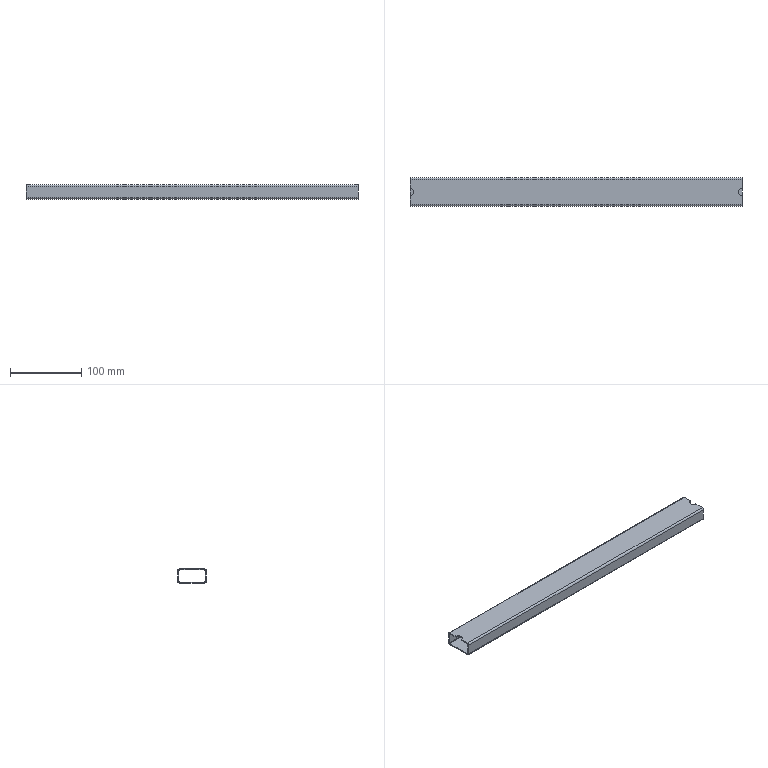Part | STEP file | 6150505 | 1 solid | 20 faces | box 465 x 40 x 20 mm | volume 77302 mm3 | plane 10 | cylinder 10 | commonest cylinder face diameters 2 x4 5 x4 10 x2
STEP:
#1=CARTESIAN_POINT('',(232.5,-5.,10.));
#2=VERTEX_POINT('',#1);
#3=CARTESIAN_POINT('',(232.5,-17.5,10.));
#4=VERTEX_POINT('',#3);
#5=CARTESIAN_POINT('',(232.5,20.,10.));
#6=DIRECTION('',(0.,-1.,0.));
#7=VECTOR('',#6,1000.);
#8=LINE('',#5,#7);
#9=EDGE_CURVE('',#2,#4,#8,.T.);
#10=ORIENTED_EDGE('',*,*,#9,.F.);
#11=CARTESIAN_POINT('',(232.5,5.,10.));
#12=VERTEX_POINT('',#11);
#13=CARTESIAN_POINT('',(232.5,0.,10.));
#14=DIRECTION('',(0.,0.,1.));
#15=DIRECTION('',(-1.,0.,0.));
#16=AXIS2_PLACEMENT_3D('',#13,#14,#15);
#17=CIRCLE('',#16,5.);
#18=EDGE_CURVE('',#12,#2,#17,.T.);
#19=ORIENTED_EDGE('',*,*,#18,.F.);
#20=CARTESIAN_POINT('',(232.5,17.5,10.));
#21=VERTEX_POINT('',#20);
#22=CARTESIAN_POINT('',(232.5,20.,10.));
#23=DIRECTION('',(0.,-1.,0.));
#24=VECTOR('',#23,1000.);
#25=LINE('',#22,#24);
#26=EDGE_CURVE('',#21,#12,#25,.T.);
#27=ORIENTED_EDGE('',*,*,#26,.F.);
#28=CARTESIAN_POINT('',(-232.5,17.5,10.));
#29=VERTEX_POINT('',#28);
#30=CARTESIAN_POINT('',(232.5,17.5,10.));
#31=DIRECTION('',(-1.,0.,0.));
#32=VECTOR('',#31,1000.);
#33=LINE('',#30,#32);
#34=EDGE_CURVE('',#21,#29,#33,.T.);
#35=ORIENTED_EDGE('',*,*,#34,.T.);
#36=CARTESIAN_POINT('',(-232.5,5.,10.));
#37=VERTEX_POINT('',#36);
#38=CARTESIAN_POINT('',(-232.5,20.,10.));
#39=DIRECTION('',(0.,-1.,0.));
#40=VECTOR('',#39,1000.);
#41=LINE('',#38,#40);
#42=EDGE_CURVE('',#29,#37,#41,.T.);
#43=ORIENTED_EDGE('',*,*,#42,.T.);
#44=CARTESIAN_POINT('',(-232.5,-5.,10.));
#45=VERTEX_POINT('',#44);
#46=CARTESIAN_POINT('',(-232.5,0.,10.));
#47=DIRECTION('',(0.,0.,1.));
#48=DIRECTION('',(1.,0.,0.));
#49=AXIS2_PLACEMENT_3D('',#46,#47,#48);
#50=CIRCLE('',#49,5.);
#51=EDGE_CURVE('',#45,#37,#50,.T.);
#52=ORIENTED_EDGE('',*,*,#51,.F.);
#53=CARTESIAN_POINT('',(-232.5,-17.5,10.));
#54=VERTEX_POINT('',#53);
#55=CARTESIAN_POINT('',(-232.5,20.,10.));
#56=DIRECTION('',(0.,-1.,0.));
#57=VECTOR('',#56,1000.);
#58=LINE('',#55,#57);
#59=EDGE_CURVE('',#45,#54,#58,.T.);
#60=ORIENTED_EDGE('',*,*,#59,.T.);
#61=CARTESIAN_POINT('',(232.5,-17.5,10.));
#62=DIRECTION('',(1.,0.,0.));
#63=VECTOR('',#62,1000.);
#64=LINE('',#61,#63);
#65=EDGE_CURVE('',#54,#4,#64,.T.);
#66=ORIENTED_EDGE('',*,*,#65,.T.);
#67=EDGE_LOOP('',(#10,#19,#27,#35,#43,#52,#60,#66));
#68=FACE_OUTER_BOUND('',#67,.T.);
#69=CARTESIAN_POINT('',(232.5,20.,10.));
#70=DIRECTION('',(0.,0.,-1.));
#71=DIRECTION('',(0.,1.,0.));
#72=AXIS2_PLACEMENT_3D('',#69,#70,#71);
#73=PLANE('',#72);
#74=ADVANCED_FACE('',(#68),#73,.F.);
#75=CARTESIAN_POINT('',(232.5,-20.,7.5));
#76=VERTEX_POINT('',#75);
#77=CARTESIAN_POINT('',(232.5,-20.,-7.5));
#78=VERTEX_POINT('',#77);
#79=CARTESIAN_POINT('',(232.5,-20.,10.));
#80=DIRECTION('',(0.,0.,-1.));
#81=VECTOR('',#80,1000.);
#82=LINE('',#79,#81);
#83=EDGE_CURVE('',#76,#78,#82,.T.);
#84=ORIENTED_EDGE('',*,*,#83,.F.);
#85=CARTESIAN_POINT('',(-232.5,-20.,7.5));
#86=VERTEX_POINT('',#85);
#87=CARTESIAN_POINT('',(232.5,-20.,7.5));
#88=DIRECTION('',(-1.,0.,0.));
#89=VECTOR('',#88,1000.);
#90=LINE('',#87,#89);
#91=EDGE_CURVE('',#76,#86,#90,.T.);
#92=ORIENTED_EDGE('',*,*,#91,.T.);
#93=CARTESIAN_POINT('',(-232.5,-20.,-7.5));
#94=VERTEX_POINT('',#93);
#95=CARTESIAN_POINT('',(-232.5,-20.,10.));
#96=DIRECTION('',(0.,0.,-1.));
#97=VECTOR('',#96,1000.);
#98=LINE('',#95,#97);
#99=EDGE_CURVE('',#86,#94,#98,.T.);
#100=ORIENTED_EDGE('',*,*,#99,.T.);
#101=CARTESIAN_POINT('',(232.5,-20.,-7.5));
#102=DIRECTION('',(1.,0.,0.));
#103=VECTOR('',#102,1000.);
#104=LINE('',#101,#103);
#105=EDGE_CURVE('',#94,#78,#104,.T.);
#106=ORIENTED_EDGE('',*,*,#105,.T.);
#107=EDGE_LOOP('',(#84,#92,#100,#106));
#108=FACE_OUTER_BOUND('',#107,.T.);
#109=CARTESIAN_POINT('',(232.5,-20.,10.));
#110=DIRECTION('',(0.,1.,0.));
#111=DIRECTION('',(0.,0.,1.));
#112=AXIS2_PLACEMENT_3D('',#109,#110,#111);
#113=PLANE('',#112);
#114=ADVANCED_FACE('',(#108),#113,.F.);
#115=CARTESIAN_POINT('',(232.5,-17.5,-10.));
#116=VERTEX_POINT('',#115);
#117=CARTESIAN_POINT('',(232.5,17.5,-10.));
#118=VERTEX_POINT('',#117);
#119=CARTESIAN_POINT('',(232.5,20.,-10.));
#120=DIRECTION('',(0.,1.,0.));
#121=VECTOR('',#120,1000.);
#122=LINE('',#119,#121);
#123=EDGE_CURVE('',#116,#118,#122,.T.);
#124=ORIENTED_EDGE('',*,*,#123,.F.);
#125=CARTESIAN_POINT('',(-232.5,-17.5,-10.));
#126=VERTEX_POINT('',#125);
#127=CARTESIAN_POINT('',(232.5,-17.5,-10.));
#128=DIRECTION('',(-1.,0.,0.));
#129=VECTOR('',#128,1000.);
#130=LINE('',#127,#129);
#131=EDGE_CURVE('',#116,#126,#130,.T.);
#132=ORIENTED_EDGE('',*,*,#131,.T.);
#133=CARTESIAN_POINT('',(-232.5,17.5,-10.));
#134=VERTEX_POINT('',#133);
#135=CARTESIAN_POINT('',(-232.5,20.,-10.));
#136=DIRECTION('',(0.,1.,0.));
#137=VECTOR('',#136,1000.);
#138=LINE('',#135,#137);
#139=EDGE_CURVE('',#126,#134,#138,.T.);
#140=ORIENTED_EDGE('',*,*,#139,.T.);
#141=CARTESIAN_POINT('',(232.5,17.5,-10.));
#142=DIRECTION('',(1.,0.,0.));
#143=VECTOR('',#142,1000.);
#144=LINE('',#141,#143);
#145=EDGE_CURVE('',#134,#118,#144,.T.);
#146=ORIENTED_EDGE('',*,*,#145,.T.);
#147=EDGE_LOOP('',(#124,#132,#140,#146));
#148=FACE_OUTER_BOUND('',#147,.T.);
#149=CARTESIAN_POINT('',(232.5,20.,-10.));
#150=DIRECTION('',(0.,0.,1.));
#151=DIRECTION('',(0.,-1.,0.));
#152=AXIS2_PLACEMENT_3D('',#149,#150,#151);
#153=PLANE('',#152);
#154=ADVANCED_FACE('',(#148),#153,.F.);
#155=CARTESIAN_POINT('',(232.5,20.,-7.5));
#156=VERTEX_POINT('',#155);
#157=CARTESIAN_POINT('',(232.5,20.,7.5));
#158=VERTEX_POINT('',#157);
#159=CARTESIAN_POINT('',(232.5,20.,10.));
#160=DIRECTION('',(0.,0.,1.));
#161=VECTOR('',#160,1000.);
#162=LINE('',#159,#161);
#163=EDGE_CURVE('',#156,#158,#162,.T.);
#164=ORIENTED_EDGE('',*,*,#163,.F.);
#165=CARTESIAN_POINT('',(-232.5,20.,-7.5));
#166=VERTEX_POINT('',#165);
#167=CARTESIAN_POINT('',(232.5,20.,-7.5));
#168=DIRECTION('',(-1.,0.,0.));
#169=VECTOR('',#168,1000.);
#170=LINE('',#167,#169);
#171=EDGE_CURVE('',#156,#166,#170,.T.);
#172=ORIENTED_EDGE('',*,*,#171,.T.);
#173=CARTESIAN_POINT('',(-232.5,20.,7.5));
#174=VERTEX_POINT('',#173);
#175=CARTESIAN_POINT('',(-232.5,20.,10.));
#176=DIRECTION('',(0.,0.,1.));
#177=VECTOR('',#176,1000.);
#178=LINE('',#175,#177);
#179=EDGE_CURVE('',#166,#174,#178,.T.);
#180=ORIENTED_EDGE('',*,*,#179,.T.);
#181=CARTESIAN_POINT('',(232.5,20.,7.5));
#182=DIRECTION('',(1.,0.,0.));
#183=VECTOR('',#182,1000.);
#184=LINE('',#181,#183);
#185=EDGE_CURVE('',#174,#158,#184,.T.);
#186=ORIENTED_EDGE('',*,*,#185,.T.);
#187=EDGE_LOOP('',(#164,#172,#180,#186));
#188=FACE_OUTER_BOUND('',#187,.T.);
#189=CARTESIAN_POINT('',(232.5,20.,10.));
#190=DIRECTION('',(0.,-1.,0.));
#191=DIRECTION('',(0.,0.,-1.));
#192=AXIS2_PLACEMENT_3D('',#189,#190,#191);
#193=PLANE('',#192);
#194=ADVANCED_FACE('',(#188),#193,.F.);
#195=CARTESIAN_POINT('',(232.5,5.,8.5));
#196=VERTEX_POINT('',#195);
#197=CARTESIAN_POINT('',(232.5,5.,5.));
#198=DIRECTION('',(0.,0.,1.));
#199=VECTOR('',#198,1000.);
#200=LINE('',#197,#199);
#201=EDGE_CURVE('',#196,#12,#200,.T.);
#202=ORIENTED_EDGE('',*,*,#201,.F.);
#203=CARTESIAN_POINT('',(232.5,17.5,8.5));
#204=VERTEX_POINT('',#203);
#205=CARTESIAN_POINT('',(232.5,20.,8.5));
#206=DIRECTION('',(0.,-1.,0.));
#207=VECTOR('',#206,1000.);
#208=LINE('',#205,#207);
#209=EDGE_CURVE('',#204,#196,#208,.T.);
#210=ORIENTED_EDGE('',*,*,#209,.F.);
#211=CARTESIAN_POINT('',(232.5,18.5,7.5));
#212=VERTEX_POINT('',#211);
#213=CARTESIAN_POINT('',(232.5,17.5,7.5));
#214=DIRECTION('',(1.,0.,0.));
#215=DIRECTION('',(0.,0.,-1.));
#216=AXIS2_PLACEMENT_3D('',#213,#214,#215);
#217=CIRCLE('',#216,1.);
#218=EDGE_CURVE('',#212,#204,#217,.T.);
#219=ORIENTED_EDGE('',*,*,#218,.F.);
#220=CARTESIAN_POINT('',(232.5,18.5,-7.5));
#221=VERTEX_POINT('',#220);
#222=CARTESIAN_POINT('',(232.5,18.5,10.));
#223=DIRECTION('',(0.,0.,1.));
#224=VECTOR('',#223,1000.);
#225=LINE('',#222,#224);
#226=EDGE_CURVE('',#221,#212,#225,.T.);
#227=ORIENTED_EDGE('',*,*,#226,.F.);
#228=CARTESIAN_POINT('',(232.5,17.5,-8.5));
#229=VERTEX_POINT('',#228);
#230=CARTESIAN_POINT('',(232.5,17.5,-7.5));
#231=DIRECTION('',(1.,0.,0.));
#232=DIRECTION('',(0.,0.,-1.));
#233=AXIS2_PLACEMENT_3D('',#230,#231,#232);
#234=CIRCLE('',#233,1.);
#235=EDGE_CURVE('',#229,#221,#234,.T.);
#236=ORIENTED_EDGE('',*,*,#235,.F.);
#237=CARTESIAN_POINT('',(232.5,-17.5,-8.5));
#238=VERTEX_POINT('',#237);
#239=CARTESIAN_POINT('',(232.5,20.,-8.5));
#240=DIRECTION('',(0.,1.,0.));
#241=VECTOR('',#240,1000.);
#242=LINE('',#239,#241);
#243=EDGE_CURVE('',#238,#229,#242,.T.);
#244=ORIENTED_EDGE('',*,*,#243,.F.);
#245=CARTESIAN_POINT('',(232.5,-18.5,-7.5));
#246=VERTEX_POINT('',#245);
#247=CARTESIAN_POINT('',(232.5,-17.5,-7.5));
#248=DIRECTION('',(1.,0.,0.));
#249=DIRECTION('',(0.,0.,-1.));
#250=AXIS2_PLACEMENT_3D('',#247,#248,#249);
#251=CIRCLE('',#250,1.);
#252=EDGE_CURVE('',#246,#238,#251,.T.);
#253=ORIENTED_EDGE('',*,*,#252,.F.);
#254=CARTESIAN_POINT('',(232.5,-18.5,7.5));
#255=VERTEX_POINT('',#254);
#256=CARTESIAN_POINT('',(232.5,-18.5,10.));
#257=DIRECTION('',(0.,0.,-1.));
#258=VECTOR('',#257,1000.);
#259=LINE('',#256,#258);
#260=EDGE_CURVE('',#255,#246,#259,.T.);
#261=ORIENTED_EDGE('',*,*,#260,.F.);
#262=CARTESIAN_POINT('',(232.5,-17.5,8.5));
#263=VERTEX_POINT('',#262);
#264=CARTESIAN_POINT('',(232.5,-17.5,7.5));
#265=DIRECTION('',(1.,0.,0.));
#266=DIRECTION('',(0.,0.,-1.));
#267=AXIS2_PLACEMENT_3D('',#264,#265,#266);
#268=CIRCLE('',#267,1.);
#269=EDGE_CURVE('',#263,#255,#268,.T.);
#270=ORIENTED_EDGE('',*,*,#269,.F.);
#271=CARTESIAN_POINT('',(232.5,-5.,8.5));
#272=VERTEX_POINT('',#271);
#273=CARTESIAN_POINT('',(232.5,20.,8.5));
#274=DIRECTION('',(0.,-1.,0.));
#275=VECTOR('',#274,1000.);
#276=LINE('',#273,#275);
#277=EDGE_CURVE('',#272,#263,#276,.T.);
#278=ORIENTED_EDGE('',*,*,#277,.F.);
#279=CARTESIAN_POINT('',(232.5,-5.,5.));
#280=DIRECTION('',(0.,0.,-1.));
#281=VECTOR('',#280,1000.);
#282=LINE('',#279,#281);
#283=EDGE_CURVE('',#2,#272,#282,.T.);
#284=ORIENTED_EDGE('',*,*,#283,.F.);
#285=ORIENTED_EDGE('',*,*,#9,.T.);
#286=CARTESIAN_POINT('',(232.5,-17.5,7.5));
#287=DIRECTION('',(1.,0.,0.));
#288=DIRECTION('',(0.,0.,-1.));
#289=AXIS2_PLACEMENT_3D('',#286,#287,#288);
#290=CIRCLE('',#289,2.5);
#291=EDGE_CURVE('',#4,#76,#290,.T.);
#292=ORIENTED_EDGE('',*,*,#291,.T.);
#293=ORIENTED_EDGE('',*,*,#83,.T.);
#294=CARTESIAN_POINT('',(232.5,-17.5,-7.5));
#295=DIRECTION('',(1.,0.,0.));
#296=DIRECTION('',(0.,0.,-1.));
#297=AXIS2_PLACEMENT_3D('',#294,#295,#296);
#298=CIRCLE('',#297,2.5);
#299=EDGE_CURVE('',#78,#116,#298,.T.);
#300=ORIENTED_EDGE('',*,*,#299,.T.);
#301=ORIENTED_EDGE('',*,*,#123,.T.);
#302=CARTESIAN_POINT('',(232.5,17.5,-7.5));
#303=DIRECTION('',(1.,0.,0.));
#304=DIRECTION('',(0.,0.,-1.));
#305=AXIS2_PLACEMENT_3D('',#302,#303,#304);
#306=CIRCLE('',#305,2.5);
#307=EDGE_CURVE('',#118,#156,#306,.T.);
#308=ORIENTED_EDGE('',*,*,#307,.T.);
#309=ORIENTED_EDGE('',*,*,#163,.T.);
#310=CARTESIAN_POINT('',(232.5,17.5,7.5));
#311=DIRECTION('',(1.,0.,0.));
#312=DIRECTION('',(0.,0.,-1.));
#313=AXIS2_PLACEMENT_3D('',#310,#311,#312);
#314=CIRCLE('',#313,2.5);
#315=EDGE_CURVE('',#158,#21,#314,.T.);
#316=ORIENTED_EDGE('',*,*,#315,.T.);
#317=ORIENTED_EDGE('',*,*,#26,.T.);
#318=EDGE_LOOP('',(#202,#210,#219,#227,#236,#244,#253,#261,#270,#278,#284,#285,#292,#293,#300,#301,#308,#309,#316,#317));
#319=FACE_OUTER_BOUND('',#318,.T.);
#320=CARTESIAN_POINT('',(232.5,-20.,10.));
#321=DIRECTION('',(1.,0.,0.));
#322=DIRECTION('',(0.,0.,-1.));
#323=AXIS2_PLACEMENT_3D('',#320,#321,#322);
#324=PLANE('',#323);
#325=ADVANCED_FACE('',(#319),#324,.T.);
#326=CARTESIAN_POINT('',(-232.5,17.5,8.5));
#327=VERTEX_POINT('',#326);
#328=CARTESIAN_POINT('',(-232.5,5.,8.5));
#329=VERTEX_POINT('',#328);
#330=CARTESIAN_POINT('',(-232.5,20.,8.5));
#331=DIRECTION('',(0.,-1.,0.));
#332=VECTOR('',#331,1000.);
#333=LINE('',#330,#332);
#334=EDGE_CURVE('',#327,#329,#333,.T.);
#335=ORIENTED_EDGE('',*,*,#334,.T.);
#336=CARTESIAN_POINT('',(-232.5,5.,5.));
#337=DIRECTION('',(0.,0.,1.));
#338=VECTOR('',#337,1000.);
#339=LINE('',#336,#338);
#340=EDGE_CURVE('',#329,#37,#339,.T.);
#341=ORIENTED_EDGE('',*,*,#340,.T.);
#342=ORIENTED_EDGE('',*,*,#42,.F.);
#343=CARTESIAN_POINT('',(-232.5,17.5,7.5));
#344=DIRECTION('',(-1.,0.,0.));
#345=DIRECTION('',(0.,0.,-1.));
#346=AXIS2_PLACEMENT_3D('',#343,#344,#345);
#347=CIRCLE('',#346,2.5);
#348=EDGE_CURVE('',#29,#174,#347,.T.);
#349=ORIENTED_EDGE('',*,*,#348,.T.);
#350=ORIENTED_EDGE('',*,*,#179,.F.);
#351=CARTESIAN_POINT('',(-232.5,17.5,-7.5));
#352=DIRECTION('',(-1.,0.,0.));
#353=DIRECTION('',(0.,0.,-1.));
#354=AXIS2_PLACEMENT_3D('',#351,#352,#353);
#355=CIRCLE('',#354,2.5);
#356=EDGE_CURVE('',#166,#134,#355,.T.);
#357=ORIENTED_EDGE('',*,*,#356,.T.);
#358=ORIENTED_EDGE('',*,*,#139,.F.);
#359=CARTESIAN_POINT('',(-232.5,-17.5,-7.5));
#360=DIRECTION('',(-1.,0.,0.));
#361=DIRECTION('',(0.,0.,-1.));
#362=AXIS2_PLACEMENT_3D('',#359,#360,#361);
#363=CIRCLE('',#362,2.5);
#364=EDGE_CURVE('',#126,#94,#363,.T.);
#365=ORIENTED_EDGE('',*,*,#364,.T.);
#366=ORIENTED_EDGE('',*,*,#99,.F.);
#367=CARTESIAN_POINT('',(-232.5,-17.5,7.5));
#368=DIRECTION('',(-1.,0.,0.));
#369=DIRECTION('',(0.,0.,-1.));
#370=AXIS2_PLACEMENT_3D('',#367,#368,#369);
#371=CIRCLE('',#370,2.5);
#372=EDGE_CURVE('',#86,#54,#371,.T.);
#373=ORIENTED_EDGE('',*,*,#372,.T.);
#374=ORIENTED_EDGE('',*,*,#59,.F.);
#375=CARTESIAN_POINT('',(-232.5,-5.,8.5));
#376=VERTEX_POINT('',#375);
#377=CARTESIAN_POINT('',(-232.5,-5.,5.));
#378=DIRECTION('',(0.,0.,-1.));
#379=VECTOR('',#378,1000.);
#380=LINE('',#377,#379);
#381=EDGE_CURVE('',#45,#376,#380,.T.);
#382=ORIENTED_EDGE('',*,*,#381,.T.);
#383=CARTESIAN_POINT('',(-232.5,-17.5,8.5));
#384=VERTEX_POINT('',#383);
#385=CARTESIAN_POINT('',(-232.5,20.,8.5));
#386=DIRECTION('',(0.,-1.,0.));
#387=VECTOR('',#386,1000.);
#388=LINE('',#385,#387);
#389=EDGE_CURVE('',#376,#384,#388,.T.);
#390=ORIENTED_EDGE('',*,*,#389,.T.);
#391=CARTESIAN_POINT('',(-232.5,-18.5,7.5));
#392=VERTEX_POINT('',#391);
#393=CARTESIAN_POINT('',(-232.5,-17.5,7.5));
#394=DIRECTION('',(-1.,0.,0.));
#395=DIRECTION('',(0.,0.,-1.));
#396=AXIS2_PLACEMENT_3D('',#393,#394,#395);
#397=CIRCLE('',#396,1.);
#398=EDGE_CURVE('',#392,#384,#397,.T.);
#399=ORIENTED_EDGE('',*,*,#398,.F.);
#400=CARTESIAN_POINT('',(-232.5,-18.5,-7.5));
#401=VERTEX_POINT('',#400);
#402=CARTESIAN_POINT('',(-232.5,-18.5,10.));
#403=DIRECTION('',(0.,0.,-1.));
#404=VECTOR('',#403,1000.);
#405=LINE('',#402,#404);
#406=EDGE_CURVE('',#392,#401,#405,.T.);
#407=ORIENTED_EDGE('',*,*,#406,.T.);
#408=CARTESIAN_POINT('',(-232.5,-17.5,-8.5));
#409=VERTEX_POINT('',#408);
#410=CARTESIAN_POINT('',(-232.5,-17.5,-7.5));
#411=DIRECTION('',(-1.,0.,0.));
#412=DIRECTION('',(0.,0.,-1.));
#413=AXIS2_PLACEMENT_3D('',#410,#411,#412);
#414=CIRCLE('',#413,1.);
#415=EDGE_CURVE('',#409,#401,#414,.T.);
#416=ORIENTED_EDGE('',*,*,#415,.F.);
#417=CARTESIAN_POINT('',(-232.5,17.5,-8.5));
#418=VERTEX_POINT('',#417);
#419=CARTESIAN_POINT('',(-232.5,20.,-8.5));
#420=DIRECTION('',(0.,1.,0.));
#421=VECTOR('',#420,1000.);
#422=LINE('',#419,#421);
#423=EDGE_CURVE('',#409,#418,#422,.T.);
#424=ORIENTED_EDGE('',*,*,#423,.T.);
#425=CARTESIAN_POINT('',(-232.5,18.5,-7.5));
#426=VERTEX_POINT('',#425);
#427=CARTESIAN_POINT('',(-232.5,17.5,-7.5));
#428=DIRECTION('',(-1.,0.,0.));
#429=DIRECTION('',(0.,0.,-1.));
#430=AXIS2_PLACEMENT_3D('',#427,#428,#429);
#431=CIRCLE('',#430,1.);
#432=EDGE_CURVE('',#426,#418,#431,.T.);
#433=ORIENTED_EDGE('',*,*,#432,.F.);
#434=CARTESIAN_POINT('',(-232.5,18.5,7.5));
#435=VERTEX_POINT('',#434);
#436=CARTESIAN_POINT('',(-232.5,18.5,10.));
#437=DIRECTION('',(0.,0.,1.));
#438=VECTOR('',#437,1000.);
#439=LINE('',#436,#438);
#440=EDGE_CURVE('',#426,#435,#439,.T.);
#441=ORIENTED_EDGE('',*,*,#440,.T.);
#442=CARTESIAN_POINT('',(-232.5,17.5,7.5));
#443=DIRECTION('',(-1.,0.,0.));
#444=DIRECTION('',(0.,0.,-1.));
#445=AXIS2_PLACEMENT_3D('',#442,#443,#444);
#446=CIRCLE('',#445,1.);
#447=EDGE_CURVE('',#327,#435,#446,.T.);
#448=ORIENTED_EDGE('',*,*,#447,.F.);
#449=EDGE_LOOP('',(#335,#341,#342,#349,#350,#357,#358,#365,#366,#373,#374,#382,#390,#399,#407,#416,#424,#433,#441,#448));
#450=FACE_OUTER_BOUND('',#449,.T.);
#451=CARTESIAN_POINT('',(-232.5,-20.,10.));
#452=DIRECTION('',(1.,0.,0.));
#453=DIRECTION('',(0.,0.,-1.));
#454=AXIS2_PLACEMENT_3D('',#451,#452,#453);
#455=PLANE('',#454);
#456=ADVANCED_FACE('',(#450),#455,.F.);
#457=ORIENTED_EDGE('',*,*,#291,.F.);
#458=ORIENTED_EDGE('',*,*,#65,.F.);
#459=ORIENTED_EDGE('',*,*,#372,.F.);
#460=ORIENTED_EDGE('',*,*,#91,.F.);
#461=EDGE_LOOP('',(#457,#458,#459,#460));
#462=FACE_OUTER_BOUND('',#461,.T.);
#463=CARTESIAN_POINT('',(232.5,-17.5,7.5));
#464=DIRECTION('',(-1.,0.,0.));
#465=DIRECTION('',(0.,0.,1.));
#466=AXIS2_PLACEMENT_3D('',#463,#464,#465);
#467=CYLINDRICAL_SURFACE('',#466,2.5);
#468=ADVANCED_FACE('',(#462),#467,.T.);
#469=ORIENTED_EDGE('',*,*,#299,.F.);
#470=ORIENTED_EDGE('',*,*,#105,.F.);
#471=ORIENTED_EDGE('',*,*,#364,.F.);
#472=ORIENTED_EDGE('',*,*,#131,.F.);
#473=EDGE_LOOP('',(#469,#470,#471,#472));
#474=FACE_OUTER_BOUND('',#473,.T.);
#475=CARTESIAN_POINT('',(232.5,-17.5,-7.5));
#476=DIRECTION('',(-1.,0.,0.));
#477=DIRECTION('',(0.,0.,1.));
#478=AXIS2_PLACEMENT_3D('',#475,#476,#477);
#479=CYLINDRICAL_SURFACE('',#478,2.5);
#480=ADVANCED_FACE('',(#474),#479,.T.);
#481=ORIENTED_EDGE('',*,*,#307,.F.);
#482=ORIENTED_EDGE('',*,*,#145,.F.);
#483=ORIENTED_EDGE('',*,*,#356,.F.);
#484=ORIENTED_EDGE('',*,*,#171,.F.);
#485=EDGE_LOOP('',(#481,#482,#483,#484));
#486=FACE_OUTER_BOUND('',#485,.T.);
#487=CARTESIAN_POINT('',(232.5,17.5,-7.5));
#488=DIRECTION('',(-1.,0.,0.));
#489=DIRECTION('',(0.,0.,1.));
#490=AXIS2_PLACEMENT_3D('',#487,#488,#489);
#491=CYLINDRICAL_SURFACE('',#490,2.5);
#492=ADVANCED_FACE('',(#486),#491,.T.);
#493=ORIENTED_EDGE('',*,*,#315,.F.);
#494=ORIENTED_EDGE('',*,*,#185,.F.);
#495=ORIENTED_EDGE('',*,*,#348,.F.);
#496=ORIENTED_EDGE('',*,*,#34,.F.);
#497=EDGE_LOOP('',(#493,#494,#495,#496));
#498=FACE_OUTER_BOUND('',#497,.T.);
#499=CARTESIAN_POINT('',(232.5,17.5,7.5));
#500=DIRECTION('',(-1.,0.,0.));
#501=DIRECTION('',(0.,0.,1.));
#502=AXIS2_PLACEMENT_3D('',#499,#500,#501);
#503=CYLINDRICAL_SURFACE('',#502,2.5);
#504=ADVANCED_FACE('',(#498),#503,.T.);
#505=CARTESIAN_POINT('',(232.5,0.,8.5));
#506=DIRECTION('',(0.,0.,-1.));
#507=DIRECTION('',(0.,1.,0.));
#508=AXIS2_PLACEMENT_3D('',#505,#506,#507);
#509=CIRCLE('',#508,5.);
#510=EDGE_CURVE('',#272,#196,#509,.T.);
#511=ORIENTED_EDGE('',*,*,#510,.F.);
#512=ORIENTED_EDGE('',*,*,#277,.T.);
#513=CARTESIAN_POINT('',(232.5,-17.5,8.5));
#514=DIRECTION('',(1.,0.,0.));
#515=VECTOR('',#514,1000.);
#516=LINE('',#513,#515);
#517=EDGE_CURVE('',#384,#263,#516,.T.);
#518=ORIENTED_EDGE('',*,*,#517,.F.);
#519=ORIENTED_EDGE('',*,*,#389,.F.);
#520=CARTESIAN_POINT('',(-232.5,0.,8.5));
#521=DIRECTION('',(0.,0.,-1.));
#522=DIRECTION('',(0.,1.,0.));
#523=AXIS2_PLACEMENT_3D('',#520,#521,#522);
#524=CIRCLE('',#523,5.);
#525=EDGE_CURVE('',#329,#376,#524,.T.);
#526=ORIENTED_EDGE('',*,*,#525,.F.);
#527=ORIENTED_EDGE('',*,*,#334,.F.);
#528=CARTESIAN_POINT('',(232.5,17.5,8.5));
#529=DIRECTION('',(-1.,0.,0.));
#530=VECTOR('',#529,1000.);
#531=LINE('',#528,#530);
#532=EDGE_CURVE('',#204,#327,#531,.T.);
#533=ORIENTED_EDGE('',*,*,#532,.F.);
#534=ORIENTED_EDGE('',*,*,#209,.T.);
#535=EDGE_LOOP('',(#511,#512,#518,#519,#526,#527,#533,#534));
#536=FACE_OUTER_BOUND('',#535,.T.);
#537=CARTESIAN_POINT('',(232.5,20.,8.5));
#538=DIRECTION('',(0.,0.,-1.));
#539=DIRECTION('',(0.,1.,0.));
#540=AXIS2_PLACEMENT_3D('',#537,#538,#539);
#541=PLANE('',#540);
#542=ADVANCED_FACE('',(#536),#541,.T.);
#543=ORIENTED_EDGE('',*,*,#260,.T.);
#544=CARTESIAN_POINT('',(232.5,-18.5,-7.5));
#545=DIRECTION('',(1.,0.,0.));
#546=VECTOR('',#545,1000.);
#547=LINE('',#544,#546);
#548=EDGE_CURVE('',#401,#246,#547,.T.);
#549=ORIENTED_EDGE('',*,*,#548,.F.);
#550=ORIENTED_EDGE('',*,*,#406,.F.);
#551=CARTESIAN_POINT('',(232.5,-18.5,7.5));
#552=DIRECTION('',(-1.,0.,0.));
#553=VECTOR('',#552,1000.);
#554=LINE('',#551,#553);
#555=EDGE_CURVE('',#255,#392,#554,.T.);
#556=ORIENTED_EDGE('',*,*,#555,.F.);
#557=EDGE_LOOP('',(#543,#549,#550,#556));
#558=FACE_OUTER_BOUND('',#557,.T.);
#559=CARTESIAN_POINT('',(232.5,-18.5,10.));
#560=DIRECTION('',(0.,1.,0.));
#561=DIRECTION('',(0.,0.,1.));
#562=AXIS2_PLACEMENT_3D('',#559,#560,#561);
#563=PLANE('',#562);
#564=ADVANCED_FACE('',(#558),#563,.T.);
#565=ORIENTED_EDGE('',*,*,#243,.T.);
#566=CARTESIAN_POINT('',(232.5,17.5,-8.5));
#567=DIRECTION('',(1.,0.,0.));
#568=VECTOR('',#567,1000.);
#569=LINE('',#566,#568);
#570=EDGE_CURVE('',#418,#229,#569,.T.);
#571=ORIENTED_EDGE('',*,*,#570,.F.);
#572=ORIENTED_EDGE('',*,*,#423,.F.);
#573=CARTESIAN_POINT('',(232.5,-17.5,-8.5));
#574=DIRECTION('',(-1.,0.,0.));
#575=VECTOR('',#574,1000.);
#576=LINE('',#573,#575);
#577=EDGE_CURVE('',#238,#409,#576,.T.);
#578=ORIENTED_EDGE('',*,*,#577,.F.);
#579=EDGE_LOOP('',(#565,#571,#572,#578));
#580=FACE_OUTER_BOUND('',#579,.T.);
#581=CARTESIAN_POINT('',(232.5,20.,-8.5));
#582=DIRECTION('',(0.,0.,1.));
#583=DIRECTION('',(0.,-1.,0.));
#584=AXIS2_PLACEMENT_3D('',#581,#582,#583);
#585=PLANE('',#584);
#586=ADVANCED_FACE('',(#580),#585,.T.);
#587=ORIENTED_EDGE('',*,*,#226,.T.);
#588=CARTESIAN_POINT('',(232.5,18.5,7.5));
#589=DIRECTION('',(1.,0.,0.));
#590=VECTOR('',#589,1000.);
#591=LINE('',#588,#590);
#592=EDGE_CURVE('',#435,#212,#591,.T.);
#593=ORIENTED_EDGE('',*,*,#592,.F.);
#594=ORIENTED_EDGE('',*,*,#440,.F.);
#595=CARTESIAN_POINT('',(232.5,18.5,-7.5));
#596=DIRECTION('',(-1.,0.,0.));
#597=VECTOR('',#596,1000.);
#598=LINE('',#595,#597);
#599=EDGE_CURVE('',#221,#426,#598,.T.);
#600=ORIENTED_EDGE('',*,*,#599,.F.);
#601=EDGE_LOOP('',(#587,#593,#594,#600));
#602=FACE_OUTER_BOUND('',#601,.T.);
#603=CARTESIAN_POINT('',(232.5,18.5,10.));
#604=DIRECTION('',(0.,-1.,0.));
#605=DIRECTION('',(0.,0.,-1.));
#606=AXIS2_PLACEMENT_3D('',#603,#604,#605);
#607=PLANE('',#606);
#608=ADVANCED_FACE('',(#602),#607,.T.);
#609=ORIENTED_EDGE('',*,*,#269,.T.);
#610=ORIENTED_EDGE('',*,*,#555,.T.);
#611=ORIENTED_EDGE('',*,*,#398,.T.);
#612=ORIENTED_EDGE('',*,*,#517,.T.);
#613=EDGE_LOOP('',(#609,#610,#611,#612));
#614=FACE_OUTER_BOUND('',#613,.T.);
#615=CARTESIAN_POINT('',(232.5,-17.5,7.5));
#616=DIRECTION('',(-1.,0.,0.));
#617=DIRECTION('',(0.,0.,1.));
#618=AXIS2_PLACEMENT_3D('',#615,#616,#617);
#619=CYLINDRICAL_SURFACE('',#618,1.);
#620=ADVANCED_FACE('',(#614),#619,.F.);
#621=ORIENTED_EDGE('',*,*,#252,.T.);
#622=ORIENTED_EDGE('',*,*,#577,.T.);
#623=ORIENTED_EDGE('',*,*,#415,.T.);
#624=ORIENTED_EDGE('',*,*,#548,.T.);
#625=EDGE_LOOP('',(#621,#622,#623,#624));
#626=FACE_OUTER_BOUND('',#625,.T.);
#627=CARTESIAN_POINT('',(232.5,-17.5,-7.5));
#628=DIRECTION('',(-1.,0.,0.));
#629=DIRECTION('',(0.,0.,1.));
#630=AXIS2_PLACEMENT_3D('',#627,#628,#629);
#631=CYLINDRICAL_SURFACE('',#630,1.);
#632=ADVANCED_FACE('',(#626),#631,.F.);
#633=ORIENTED_EDGE('',*,*,#235,.T.);
#634=ORIENTED_EDGE('',*,*,#599,.T.);
#635=ORIENTED_EDGE('',*,*,#432,.T.);
#636=ORIENTED_EDGE('',*,*,#570,.T.);
#637=EDGE_LOOP('',(#633,#634,#635,#636));
#638=FACE_OUTER_BOUND('',#637,.T.);
#639=CARTESIAN_POINT('',(232.5,17.5,-7.5));
#640=DIRECTION('',(-1.,0.,0.));
#641=DIRECTION('',(0.,0.,1.));
#642=AXIS2_PLACEMENT_3D('',#639,#640,#641);
#643=CYLINDRICAL_SURFACE('',#642,1.);
#644=ADVANCED_FACE('',(#638),#643,.F.);
#645=ORIENTED_EDGE('',*,*,#218,.T.);
#646=ORIENTED_EDGE('',*,*,#532,.T.);
#647=ORIENTED_EDGE('',*,*,#447,.T.);
#648=ORIENTED_EDGE('',*,*,#592,.T.);
#649=EDGE_LOOP('',(#645,#646,#647,#648));
#650=FACE_OUTER_BOUND('',#649,.T.);
#651=CARTESIAN_POINT('',(232.5,17.5,7.5));
#652=DIRECTION('',(-1.,0.,0.));
#653=DIRECTION('',(0.,0.,1.));
#654=AXIS2_PLACEMENT_3D('',#651,#652,#653);
#655=CYLINDRICAL_SURFACE('',#654,1.);
#656=ADVANCED_FACE('',(#650),#655,.F.);
#657=ORIENTED_EDGE('',*,*,#525,.T.);
#658=ORIENTED_EDGE('',*,*,#381,.F.);
#659=ORIENTED_EDGE('',*,*,#51,.T.);
#660=ORIENTED_EDGE('',*,*,#340,.F.);
#661=EDGE_LOOP('',(#657,#658,#659,#660));
#662=FACE_OUTER_BOUND('',#661,.T.);
#663=CARTESIAN_POINT('',(-232.5,0.,5.));
#664=DIRECTION('',(0.,0.,1.));
#665=DIRECTION('',(1.,0.,0.));
#666=AXIS2_PLACEMENT_3D('',#663,#664,#665);
#667=CYLINDRICAL_SURFACE('',#666,5.);
#668=ADVANCED_FACE('',(#662),#667,.F.);
#669=ORIENTED_EDGE('',*,*,#201,.T.);
#670=ORIENTED_EDGE('',*,*,#18,.T.);
#671=ORIENTED_EDGE('',*,*,#283,.T.);
#672=ORIENTED_EDGE('',*,*,#510,.T.);
#673=EDGE_LOOP('',(#669,#670,#671,#672));
#674=FACE_OUTER_BOUND('',#673,.T.);
#675=CARTESIAN_POINT('',(232.5,0.,5.));
#676=DIRECTION('',(0.,0.,1.));
#677=DIRECTION('',(1.,0.,0.));
#678=AXIS2_PLACEMENT_3D('',#675,#676,#677);
#679=CYLINDRICAL_SURFACE('',#678,5.);
#680=ADVANCED_FACE('',(#674),#679,.F.);
#681=CLOSED_SHELL('',(#74,#114,#154,#194,#325,#456,#468,#480,#492,#504,#542,#564,#586,#608,#620,#632,#644,#656,#668,#680));
#682=MANIFOLD_SOLID_BREP('',#681);
#683=CARTESIAN_POINT('',(0.,0.,0.));
#684=DIRECTION('',(0.,0.,1.));
#685=DIRECTION('',(1.,0.,0.));
#686=AXIS2_PLACEMENT_3D('',#683,#684,#685);
#687=(LENGTH_UNIT()NAMED_UNIT(*)SI_UNIT(.MILLI.,.METRE.));
#688=UNCERTAINTY_MEASURE_WITH_UNIT(LENGTH_MEASURE(0.00001),#687,'','');
#689=(NAMED_UNIT(*)PLANE_ANGLE_UNIT()SI_UNIT($,.RADIAN.));
#690=(NAMED_UNIT(*)SI_UNIT($,.STERADIAN.)SOLID_ANGLE_UNIT());
#691=(GEOMETRIC_REPRESENTATION_CONTEXT(3)GLOBAL_UNCERTAINTY_ASSIGNED_CONTEXT((#688))GLOBAL_UNIT_ASSIGNED_CONTEXT((#687,#689,#690))REPRESENTATION_CONTEXT('',''));
#692=ADVANCED_BREP_SHAPE_REPRESENTATION('',(#682,#686),#691);